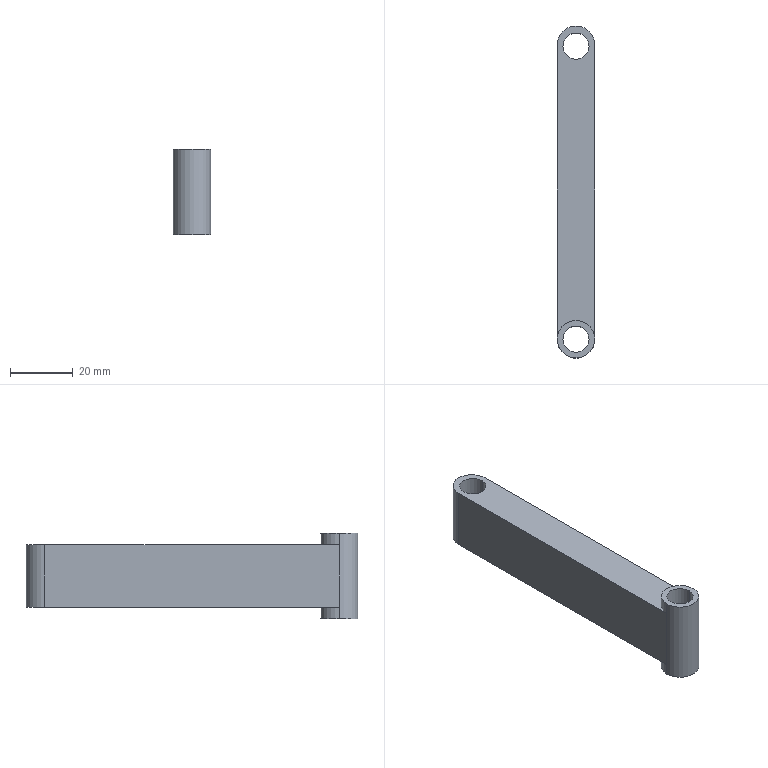Part | SolidWorks | features ICE 2, Extrusion 1, Fillet 1 | 1 solid | 15 faces | box 12 x 106 x 27.4 mm | volume 23043 mm3 | cylinder 9 | plane 6 | commonest cylinder face diameters 12 x5 8.382 x4
STEP:
#1=CARTESIAN_POINT('',(-4.191,0.,0.));
#2=VERTEX_POINT('',#1);
#3=CARTESIAN_POINT('',(4.191,0.,0.));
#4=VERTEX_POINT('',#3);
#5=CARTESIAN_POINT('',(0.,0.,0.));
#6=DIRECTION('',(0.,0.,1.));
#7=DIRECTION('',(1.,0.,0.));
#8=AXIS2_PLACEMENT_3D('',#5,#6,#7);
#9=CIRCLE('',#8,4.191);
#10=EDGE_CURVE('',#2,#4,#9,.T.);
#11=ORIENTED_EDGE('',*,*,#10,.F.);
#12=CARTESIAN_POINT('',(-4.191,0.,27.4));
#13=VERTEX_POINT('',#12);
#14=CARTESIAN_POINT('',(-4.191,0.,-36.3));
#15=DIRECTION('',(0.,0.,1.));
#16=VECTOR('',#15,1000.);
#17=LINE('',#14,#16);
#18=EDGE_CURVE('',#2,#13,#17,.T.);
#19=ORIENTED_EDGE('',*,*,#18,.T.);
#20=CARTESIAN_POINT('',(4.191,0.,27.4));
#21=VERTEX_POINT('',#20);
#22=CARTESIAN_POINT('',(0.,0.,27.4));
#23=DIRECTION('',(0.,0.,1.));
#24=DIRECTION('',(1.,0.,0.));
#25=AXIS2_PLACEMENT_3D('',#22,#23,#24);
#26=CIRCLE('',#25,4.191);
#27=EDGE_CURVE('',#13,#21,#26,.T.);
#28=ORIENTED_EDGE('',*,*,#27,.T.);
#29=CARTESIAN_POINT('',(4.191,0.,-36.3));
#30=DIRECTION('',(0.,0.,1.));
#31=VECTOR('',#30,1000.);
#32=LINE('',#29,#31);
#33=EDGE_CURVE('',#4,#21,#32,.T.);
#34=ORIENTED_EDGE('',*,*,#33,.F.);
#35=EDGE_LOOP('',(#11,#19,#28,#34));
#36=FACE_OUTER_BOUND('',#35,.T.);
#37=CARTESIAN_POINT('',(0.,0.,-36.3));
#38=DIRECTION('',(0.,0.,1.));
#39=DIRECTION('',(1.,0.,0.));
#40=AXIS2_PLACEMENT_3D('',#37,#38,#39);
#41=CYLINDRICAL_SURFACE('',#40,4.191);
#42=ADVANCED_FACE('',(#36),#41,.F.);
#43=CARTESIAN_POINT('',(-4.191,93.553,3.7));
#44=VERTEX_POINT('',#43);
#45=CARTESIAN_POINT('',(4.191,93.553,3.7));
#46=VERTEX_POINT('',#45);
#47=CARTESIAN_POINT('',(0.,93.553,3.7));
#48=DIRECTION('',(0.,0.,1.));
#49=DIRECTION('',(1.,0.,0.));
#50=AXIS2_PLACEMENT_3D('',#47,#48,#49);
#51=CIRCLE('',#50,4.191);
#52=EDGE_CURVE('',#44,#46,#51,.T.);
#53=ORIENTED_EDGE('',*,*,#52,.F.);
#54=CARTESIAN_POINT('',(-4.191,93.553,23.7));
#55=VERTEX_POINT('',#54);
#56=CARTESIAN_POINT('',(-4.191,93.553,-36.3));
#57=DIRECTION('',(0.,0.,1.));
#58=VECTOR('',#57,1000.);
#59=LINE('',#56,#58);
#60=EDGE_CURVE('',#44,#55,#59,.T.);
#61=ORIENTED_EDGE('',*,*,#60,.T.);
#62=CARTESIAN_POINT('',(4.191,93.553,23.7));
#63=VERTEX_POINT('',#62);
#64=CARTESIAN_POINT('',(0.,93.553,23.7));
#65=DIRECTION('',(0.,0.,-1.));
#66=DIRECTION('',(-1.,0.,0.));
#67=AXIS2_PLACEMENT_3D('',#64,#65,#66);
#68=CIRCLE('',#67,4.191);
#69=EDGE_CURVE('',#63,#55,#68,.T.);
#70=ORIENTED_EDGE('',*,*,#69,.F.);
#71=CARTESIAN_POINT('',(4.191,93.553,-36.3));
#72=DIRECTION('',(0.,0.,1.));
#73=VECTOR('',#72,1000.);
#74=LINE('',#71,#73);
#75=EDGE_CURVE('',#46,#63,#74,.T.);
#76=ORIENTED_EDGE('',*,*,#75,.F.);
#77=EDGE_LOOP('',(#53,#61,#70,#76));
#78=FACE_OUTER_BOUND('',#77,.T.);
#79=CARTESIAN_POINT('',(0.,93.553,-36.3));
#80=DIRECTION('',(0.,0.,1.));
#81=DIRECTION('',(1.,0.,0.));
#82=AXIS2_PLACEMENT_3D('',#79,#80,#81);
#83=CYLINDRICAL_SURFACE('',#82,4.191);
#84=ADVANCED_FACE('',(#78),#83,.F.);
#85=CARTESIAN_POINT('',(6.,0.,27.4));
#86=VERTEX_POINT('',#85);
#87=CARTESIAN_POINT('',(-6.,0.,27.4));
#88=VERTEX_POINT('',#87);
#89=CARTESIAN_POINT('',(0.,0.,27.4));
#90=DIRECTION('',(0.,0.,1.));
#91=DIRECTION('',(1.,0.,0.));
#92=AXIS2_PLACEMENT_3D('',#89,#90,#91);
#93=CIRCLE('',#92,6.);
#94=EDGE_CURVE('',#86,#88,#93,.T.);
#95=ORIENTED_EDGE('',*,*,#94,.F.);
#96=CARTESIAN_POINT('',(6.,0.,23.7));
#97=VERTEX_POINT('',#96);
#98=CARTESIAN_POINT('',(6.,0.,27.4));
#99=DIRECTION('',(0.,0.,-1.));
#100=VECTOR('',#99,1000.);
#101=LINE('',#98,#100);
#102=EDGE_CURVE('',#86,#97,#101,.T.);
#103=ORIENTED_EDGE('',*,*,#102,.T.);
#104=CARTESIAN_POINT('',(-6.,0.,23.7));
#105=VERTEX_POINT('',#104);
#106=CARTESIAN_POINT('',(0.,0.,23.7));
#107=DIRECTION('',(0.,0.,-1.));
#108=DIRECTION('',(-1.,0.,0.));
#109=AXIS2_PLACEMENT_3D('',#106,#107,#108);
#110=CIRCLE('',#109,6.);
#111=EDGE_CURVE('',#105,#97,#110,.T.);
#112=ORIENTED_EDGE('',*,*,#111,.F.);
#113=CARTESIAN_POINT('',(-6.,0.,27.4));
#114=DIRECTION('',(0.,0.,-1.));
#115=VECTOR('',#114,1000.);
#116=LINE('',#113,#115);
#117=EDGE_CURVE('',#88,#105,#116,.T.);
#118=ORIENTED_EDGE('',*,*,#117,.F.);
#119=EDGE_LOOP('',(#95,#103,#112,#118));
#120=FACE_OUTER_BOUND('',#119,.T.);
#121=CARTESIAN_POINT('',(0.,0.,27.4));
#122=DIRECTION('',(0.,0.,-1.));
#123=DIRECTION('',(-1.,0.,0.));
#124=AXIS2_PLACEMENT_3D('',#121,#122,#123);
#125=CYLINDRICAL_SURFACE('',#124,6.);
#126=ADVANCED_FACE('',(#120),#125,.T.);
#127=CARTESIAN_POINT('',(6.,0.,3.7));
#128=VERTEX_POINT('',#127);
#129=CARTESIAN_POINT('',(-6.,0.,3.7));
#130=VERTEX_POINT('',#129);
#131=CARTESIAN_POINT('',(0.,0.,3.7));
#132=DIRECTION('',(0.,0.,1.));
#133=DIRECTION('',(1.,0.,0.));
#134=AXIS2_PLACEMENT_3D('',#131,#132,#133);
#135=CIRCLE('',#134,6.);
#136=EDGE_CURVE('',#128,#130,#135,.T.);
#137=ORIENTED_EDGE('',*,*,#136,.F.);
#138=CARTESIAN_POINT('',(6.,0.,0.));
#139=VERTEX_POINT('',#138);
#140=CARTESIAN_POINT('',(6.,0.,27.4));
#141=DIRECTION('',(0.,0.,-1.));
#142=VECTOR('',#141,1000.);
#143=LINE('',#140,#142);
#144=EDGE_CURVE('',#128,#139,#143,.T.);
#145=ORIENTED_EDGE('',*,*,#144,.T.);
#146=CARTESIAN_POINT('',(-6.,0.,0.));
#147=VERTEX_POINT('',#146);
#148=CARTESIAN_POINT('',(0.,0.,0.));
#149=DIRECTION('',(0.,0.,1.));
#150=DIRECTION('',(1.,0.,0.));
#151=AXIS2_PLACEMENT_3D('',#148,#149,#150);
#152=CIRCLE('',#151,6.);
#153=EDGE_CURVE('',#139,#147,#152,.T.);
#154=ORIENTED_EDGE('',*,*,#153,.T.);
#155=CARTESIAN_POINT('',(-6.,0.,27.4));
#156=DIRECTION('',(0.,0.,-1.));
#157=VECTOR('',#156,1000.);
#158=LINE('',#155,#157);
#159=EDGE_CURVE('',#130,#147,#158,.T.);
#160=ORIENTED_EDGE('',*,*,#159,.F.);
#161=EDGE_LOOP('',(#137,#145,#154,#160));
#162=FACE_OUTER_BOUND('',#161,.T.);
#163=CARTESIAN_POINT('',(0.,0.,27.4));
#164=DIRECTION('',(0.,0.,-1.));
#165=DIRECTION('',(-1.,0.,0.));
#166=AXIS2_PLACEMENT_3D('',#163,#164,#165);
#167=CYLINDRICAL_SURFACE('',#166,6.);
#168=ADVANCED_FACE('',(#162),#167,.T.);
#169=ORIENTED_EDGE('',*,*,#102,.F.);
#170=CARTESIAN_POINT('',(0.,0.,27.4));
#171=DIRECTION('',(0.,0.,1.));
#172=DIRECTION('',(1.,0.,0.));
#173=AXIS2_PLACEMENT_3D('',#170,#171,#172);
#174=CIRCLE('',#173,6.);
#175=EDGE_CURVE('',#88,#86,#174,.T.);
#176=ORIENTED_EDGE('',*,*,#175,.F.);
#177=ORIENTED_EDGE('',*,*,#117,.T.);
#178=CARTESIAN_POINT('',(-6.,0.,23.7));
#179=DIRECTION('',(0.,0.,1.));
#180=VECTOR('',#179,1000.);
#181=LINE('',#178,#180);
#182=EDGE_CURVE('',#130,#105,#181,.T.);
#183=ORIENTED_EDGE('',*,*,#182,.F.);
#184=ORIENTED_EDGE('',*,*,#159,.T.);
#185=CARTESIAN_POINT('',(0.,0.,0.));
#186=DIRECTION('',(0.,0.,1.));
#187=DIRECTION('',(1.,0.,0.));
#188=AXIS2_PLACEMENT_3D('',#185,#186,#187);
#189=CIRCLE('',#188,6.);
#190=EDGE_CURVE('',#147,#139,#189,.T.);
#191=ORIENTED_EDGE('',*,*,#190,.T.);
#192=ORIENTED_EDGE('',*,*,#144,.F.);
#193=CARTESIAN_POINT('',(6.,0.,3.7));
#194=DIRECTION('',(0.,0.,-1.));
#195=VECTOR('',#194,1000.);
#196=LINE('',#193,#195);
#197=EDGE_CURVE('',#97,#128,#196,.T.);
#198=ORIENTED_EDGE('',*,*,#197,.F.);
#199=EDGE_LOOP('',(#169,#176,#177,#183,#184,#191,#192,#198));
#200=FACE_OUTER_BOUND('',#199,.T.);
#201=CARTESIAN_POINT('',(0.,0.,27.4));
#202=DIRECTION('',(0.,0.,-1.));
#203=DIRECTION('',(-1.,0.,0.));
#204=AXIS2_PLACEMENT_3D('',#201,#202,#203);
#205=CYLINDRICAL_SURFACE('',#204,6.);
#206=ADVANCED_FACE('',(#200),#205,.T.);
#207=CARTESIAN_POINT('',(0.,0.,27.4));
#208=DIRECTION('',(0.,0.,1.));
#209=DIRECTION('',(1.,0.,0.));
#210=AXIS2_PLACEMENT_3D('',#207,#208,#209);
#211=CIRCLE('',#210,4.191);
#212=EDGE_CURVE('',#21,#13,#211,.T.);
#213=ORIENTED_EDGE('',*,*,#212,.F.);
#214=ORIENTED_EDGE('',*,*,#27,.F.);
#215=EDGE_LOOP('',(#213,#214));
#216=FACE_BOUND('',#215,.T.);
#217=ORIENTED_EDGE('',*,*,#175,.T.);
#218=ORIENTED_EDGE('',*,*,#94,.T.);
#219=EDGE_LOOP('',(#217,#218));
#220=FACE_OUTER_BOUND('',#219,.T.);
#221=CARTESIAN_POINT('',(0.,0.,27.4));
#222=DIRECTION('',(0.,0.,1.));
#223=DIRECTION('',(1.,0.,0.));
#224=AXIS2_PLACEMENT_3D('',#221,#222,#223);
#225=PLANE('',#224);
#226=ADVANCED_FACE('',(#216,#220),#225,.T.);
#227=CARTESIAN_POINT('',(0.,0.,0.));
#228=DIRECTION('',(0.,0.,1.));
#229=DIRECTION('',(1.,0.,0.));
#230=AXIS2_PLACEMENT_3D('',#227,#228,#229);
#231=CIRCLE('',#230,4.191);
#232=EDGE_CURVE('',#4,#2,#231,.T.);
#233=ORIENTED_EDGE('',*,*,#232,.T.);
#234=ORIENTED_EDGE('',*,*,#10,.T.);
#235=EDGE_LOOP('',(#233,#234));
#236=FACE_BOUND('',#235,.T.);
#237=ORIENTED_EDGE('',*,*,#190,.F.);
#238=ORIENTED_EDGE('',*,*,#153,.F.);
#239=EDGE_LOOP('',(#237,#238));
#240=FACE_OUTER_BOUND('',#239,.T.);
#241=CARTESIAN_POINT('',(0.,0.,0.));
#242=DIRECTION('',(0.,0.,1.));
#243=DIRECTION('',(1.,0.,0.));
#244=AXIS2_PLACEMENT_3D('',#241,#242,#243);
#245=PLANE('',#244);
#246=ADVANCED_FACE('',(#236,#240),#245,.F.);
#247=ORIENTED_EDGE('',*,*,#69,.T.);
#248=CARTESIAN_POINT('',(0.,93.553,23.7));
#249=DIRECTION('',(0.,0.,-1.));
#250=DIRECTION('',(-1.,0.,0.));
#251=AXIS2_PLACEMENT_3D('',#248,#249,#250);
#252=CIRCLE('',#251,4.191);
#253=EDGE_CURVE('',#55,#63,#252,.T.);
#254=ORIENTED_EDGE('',*,*,#253,.T.);
#255=EDGE_LOOP('',(#247,#254));
#256=FACE_BOUND('',#255,.T.);
#257=CARTESIAN_POINT('',(6.,94.,23.7));
#258=VERTEX_POINT('',#257);
#259=CARTESIAN_POINT('',(6.,100.,23.7));
#260=DIRECTION('',(0.,-1.,0.));
#261=VECTOR('',#260,1000.);
#262=LINE('',#259,#261);
#263=EDGE_CURVE('',#258,#97,#262,.T.);
#264=ORIENTED_EDGE('',*,*,#263,.F.);
#265=CARTESIAN_POINT('',(0.,100.,23.7));
#266=VERTEX_POINT('',#265);
#267=CARTESIAN_POINT('',(0.,94.,23.7));
#268=DIRECTION('',(0.,0.,1.));
#269=DIRECTION('',(-1.,0.,0.));
#270=AXIS2_PLACEMENT_3D('',#267,#268,#269);
#271=CIRCLE('',#270,6.);
#272=EDGE_CURVE('',#258,#266,#271,.T.);
#273=ORIENTED_EDGE('',*,*,#272,.T.);
#274=CARTESIAN_POINT('',(-6.,94.,23.7));
#275=VERTEX_POINT('',#274);
#276=CARTESIAN_POINT('',(0.,94.,23.7));
#277=DIRECTION('',(0.,0.,1.));
#278=DIRECTION('',(-1.,0.,0.));
#279=AXIS2_PLACEMENT_3D('',#276,#277,#278);
#280=CIRCLE('',#279,6.);
#281=EDGE_CURVE('',#266,#275,#280,.T.);
#282=ORIENTED_EDGE('',*,*,#281,.T.);
#283=CARTESIAN_POINT('',(-6.,100.,23.7));
#284=DIRECTION('',(0.,-1.,0.));
#285=VECTOR('',#284,1000.);
#286=LINE('',#283,#285);
#287=EDGE_CURVE('',#275,#105,#286,.T.);
#288=ORIENTED_EDGE('',*,*,#287,.T.);
#289=ORIENTED_EDGE('',*,*,#111,.T.);
#290=EDGE_LOOP('',(#264,#273,#282,#288,#289));
#291=FACE_OUTER_BOUND('',#290,.T.);
#292=CARTESIAN_POINT('',(-6.,100.,23.7));
#293=DIRECTION('',(0.,0.,-1.));
#294=DIRECTION('',(-1.,0.,0.));
#295=AXIS2_PLACEMENT_3D('',#292,#293,#294);
#296=PLANE('',#295);
#297=ADVANCED_FACE('',(#256,#291),#296,.F.);
#298=CARTESIAN_POINT('',(6.,94.,3.7));
#299=VERTEX_POINT('',#298);
#300=CARTESIAN_POINT('',(6.,100.,3.7));
#301=DIRECTION('',(0.,-1.,0.));
#302=VECTOR('',#301,1000.);
#303=LINE('',#300,#302);
#304=EDGE_CURVE('',#299,#128,#303,.T.);
#305=ORIENTED_EDGE('',*,*,#304,.F.);
#306=CARTESIAN_POINT('',(6.,94.,3.7));
#307=DIRECTION('',(0.,0.,1.));
#308=VECTOR('',#307,1000.);
#309=LINE('',#306,#308);
#310=EDGE_CURVE('',#299,#258,#309,.T.);
#311=ORIENTED_EDGE('',*,*,#310,.T.);
#312=ORIENTED_EDGE('',*,*,#263,.T.);
#313=ORIENTED_EDGE('',*,*,#197,.T.);
#314=EDGE_LOOP('',(#305,#311,#312,#313));
#315=FACE_OUTER_BOUND('',#314,.T.);
#316=CARTESIAN_POINT('',(6.,100.,3.7));
#317=DIRECTION('',(-1.,0.,0.));
#318=DIRECTION('',(0.,0.,1.));
#319=AXIS2_PLACEMENT_3D('',#316,#317,#318);
#320=PLANE('',#319);
#321=ADVANCED_FACE('',(#315),#320,.F.);
#322=CARTESIAN_POINT('',(0.,93.553,3.7));
#323=DIRECTION('',(0.,0.,1.));
#324=DIRECTION('',(1.,0.,0.));
#325=AXIS2_PLACEMENT_3D('',#322,#323,#324);
#326=CIRCLE('',#325,4.191);
#327=EDGE_CURVE('',#46,#44,#326,.T.);
#328=ORIENTED_EDGE('',*,*,#327,.T.);
#329=ORIENTED_EDGE('',*,*,#52,.T.);
#330=EDGE_LOOP('',(#328,#329));
#331=FACE_BOUND('',#330,.T.);
#332=CARTESIAN_POINT('',(-6.,94.,3.7));
#333=VERTEX_POINT('',#332);
#334=CARTESIAN_POINT('',(0.,100.,3.7));
#335=VERTEX_POINT('',#334);
#336=CARTESIAN_POINT('',(0.,94.,3.7));
#337=DIRECTION('',(0.,0.,-1.));
#338=DIRECTION('',(1.,0.,0.));
#339=AXIS2_PLACEMENT_3D('',#336,#337,#338);
#340=CIRCLE('',#339,6.);
#341=EDGE_CURVE('',#333,#335,#340,.T.);
#342=ORIENTED_EDGE('',*,*,#341,.T.);
#343=CARTESIAN_POINT('',(0.,94.,3.7));
#344=DIRECTION('',(0.,0.,-1.));
#345=DIRECTION('',(1.,0.,0.));
#346=AXIS2_PLACEMENT_3D('',#343,#344,#345);
#347=CIRCLE('',#346,6.);
#348=EDGE_CURVE('',#335,#299,#347,.T.);
#349=ORIENTED_EDGE('',*,*,#348,.T.);
#350=ORIENTED_EDGE('',*,*,#304,.T.);
#351=ORIENTED_EDGE('',*,*,#136,.T.);
#352=CARTESIAN_POINT('',(-6.,100.,3.7));
#353=DIRECTION('',(0.,-1.,0.));
#354=VECTOR('',#353,1000.);
#355=LINE('',#352,#354);
#356=EDGE_CURVE('',#333,#130,#355,.T.);
#357=ORIENTED_EDGE('',*,*,#356,.F.);
#358=EDGE_LOOP('',(#342,#349,#350,#351,#357));
#359=FACE_OUTER_BOUND('',#358,.T.);
#360=CARTESIAN_POINT('',(-6.,100.,3.7));
#361=DIRECTION('',(0.,0.,1.));
#362=DIRECTION('',(1.,0.,0.));
#363=AXIS2_PLACEMENT_3D('',#360,#361,#362);
#364=PLANE('',#363);
#365=ADVANCED_FACE('',(#331,#359),#364,.F.);
#366=ORIENTED_EDGE('',*,*,#287,.F.);
#367=CARTESIAN_POINT('',(-6.,94.,23.7));
#368=DIRECTION('',(0.,0.,-1.));
#369=VECTOR('',#368,1000.);
#370=LINE('',#367,#369);
#371=EDGE_CURVE('',#275,#333,#370,.T.);
#372=ORIENTED_EDGE('',*,*,#371,.T.);
#373=ORIENTED_EDGE('',*,*,#356,.T.);
#374=ORIENTED_EDGE('',*,*,#182,.T.);
#375=EDGE_LOOP('',(#366,#372,#373,#374));
#376=FACE_OUTER_BOUND('',#375,.T.);
#377=CARTESIAN_POINT('',(-6.,100.,23.7));
#378=DIRECTION('',(1.,0.,0.));
#379=DIRECTION('',(0.,0.,-1.));
#380=AXIS2_PLACEMENT_3D('',#377,#378,#379);
#381=PLANE('',#380);
#382=ADVANCED_FACE('',(#376),#381,.F.);
#383=ORIENTED_EDGE('',*,*,#60,.F.);
#384=ORIENTED_EDGE('',*,*,#327,.F.);
#385=ORIENTED_EDGE('',*,*,#75,.T.);
#386=ORIENTED_EDGE('',*,*,#253,.F.);
#387=EDGE_LOOP('',(#383,#384,#385,#386));
#388=FACE_OUTER_BOUND('',#387,.T.);
#389=CARTESIAN_POINT('',(0.,93.553,-36.3));
#390=DIRECTION('',(0.,0.,1.));
#391=DIRECTION('',(1.,0.,0.));
#392=AXIS2_PLACEMENT_3D('',#389,#390,#391);
#393=CYLINDRICAL_SURFACE('',#392,4.191);
#394=ADVANCED_FACE('',(#388),#393,.F.);
#395=ORIENTED_EDGE('',*,*,#18,.F.);
#396=ORIENTED_EDGE('',*,*,#232,.F.);
#397=ORIENTED_EDGE('',*,*,#33,.T.);
#398=ORIENTED_EDGE('',*,*,#212,.T.);
#399=EDGE_LOOP('',(#395,#396,#397,#398));
#400=FACE_OUTER_BOUND('',#399,.T.);
#401=CARTESIAN_POINT('',(0.,0.,-36.3));
#402=DIRECTION('',(0.,0.,1.));
#403=DIRECTION('',(1.,0.,0.));
#404=AXIS2_PLACEMENT_3D('',#401,#402,#403);
#405=CYLINDRICAL_SURFACE('',#404,4.191);
#406=ADVANCED_FACE('',(#400),#405,.F.);
#407=ORIENTED_EDGE('',*,*,#371,.F.);
#408=ORIENTED_EDGE('',*,*,#281,.F.);
#409=CARTESIAN_POINT('',(0.,100.,0.));
#410=DIRECTION('',(0.,0.,1.));
#411=VECTOR('',#410,1000.);
#412=LINE('',#409,#411);
#413=EDGE_CURVE('',#335,#266,#412,.T.);
#414=ORIENTED_EDGE('',*,*,#413,.F.);
#415=ORIENTED_EDGE('',*,*,#341,.F.);
#416=EDGE_LOOP('',(#407,#408,#414,#415));
#417=FACE_OUTER_BOUND('',#416,.T.);
#418=CARTESIAN_POINT('',(0.,94.,0.));
#419=DIRECTION('',(0.,0.,1.));
#420=DIRECTION('',(1.,0.,0.));
#421=AXIS2_PLACEMENT_3D('',#418,#419,#420);
#422=CYLINDRICAL_SURFACE('',#421,6.);
#423=ADVANCED_FACE('',(#417),#422,.T.);
#424=ORIENTED_EDGE('',*,*,#272,.F.);
#425=ORIENTED_EDGE('',*,*,#310,.F.);
#426=ORIENTED_EDGE('',*,*,#348,.F.);
#427=ORIENTED_EDGE('',*,*,#413,.T.);
#428=EDGE_LOOP('',(#424,#425,#426,#427));
#429=FACE_OUTER_BOUND('',#428,.T.);
#430=CARTESIAN_POINT('',(0.,94.,0.));
#431=DIRECTION('',(0.,0.,-1.));
#432=DIRECTION('',(-1.,0.,0.));
#433=AXIS2_PLACEMENT_3D('',#430,#431,#432);
#434=CYLINDRICAL_SURFACE('',#433,6.);
#435=ADVANCED_FACE('',(#429),#434,.T.);
#436=CLOSED_SHELL('',(#42,#84,#126,#168,#206,#226,#246,#297,#321,#365,#382,#394,#406,#423,#435));
#437=MANIFOLD_SOLID_BREP('',#436);
#438=CARTESIAN_POINT('',(0.,0.,0.));
#439=DIRECTION('',(0.,0.,1.));
#440=DIRECTION('',(1.,0.,0.));
#441=AXIS2_PLACEMENT_3D('',#438,#439,#440);
#442=(LENGTH_UNIT()NAMED_UNIT(*)SI_UNIT(.MILLI.,.METRE.));
#443=UNCERTAINTY_MEASURE_WITH_UNIT(LENGTH_MEASURE(0.00001),#442,'','');
#444=(NAMED_UNIT(*)PLANE_ANGLE_UNIT()SI_UNIT($,.RADIAN.));
#445=(NAMED_UNIT(*)SI_UNIT($,.STERADIAN.)SOLID_ANGLE_UNIT());
#446=(GEOMETRIC_REPRESENTATION_CONTEXT(3)GLOBAL_UNCERTAINTY_ASSIGNED_CONTEXT((#443))GLOBAL_UNIT_ASSIGNED_CONTEXT((#442,#444,#445))REPRESENTATION_CONTEXT('',''));
#447=ADVANCED_BREP_SHAPE_REPRESENTATION('',(#437,#441),#446);